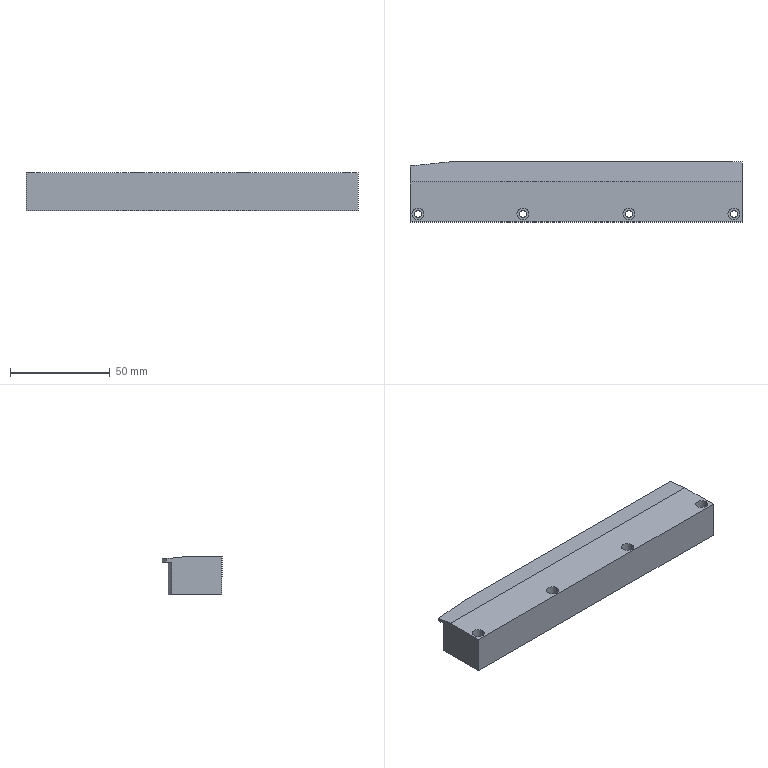Part | SolidWorks | features BaseBody 1 | 1 solid | 31 faces | box 166 x 30 x 19 mm | volume 83734 mm3 | cylinder 16 | plane 15 | commonest cylinder face diameters 3.5 x8 6 x8
STEP:
#1=CARTESIAN_POINT('',(112.721,-3.095,0.));
#2=VERTEX_POINT('',#1);
#3=CARTESIAN_POINT('',(109.221,-3.095,0.));
#4=VERTEX_POINT('',#3);
#5=CARTESIAN_POINT('',(110.971,-3.095,0.));
#6=DIRECTION('',(0.,0.,-1.));
#7=DIRECTION('',(1.,0.,0.));
#8=AXIS2_PLACEMENT_3D('',#5,#6,#7);
#9=CIRCLE('',#8,1.75);
#10=EDGE_CURVE('',#2,#4,#9,.T.);
#11=ORIENTED_EDGE('',*,*,#10,.T.);
#12=CARTESIAN_POINT('',(109.221,-3.095,9.));
#13=VERTEX_POINT('',#12);
#14=CARTESIAN_POINT('',(109.221,-3.095,-150.756));
#15=DIRECTION('',(0.,0.,1.));
#16=VECTOR('',#15,1000.);
#17=LINE('',#14,#16);
#18=EDGE_CURVE('',#4,#13,#17,.T.);
#19=ORIENTED_EDGE('',*,*,#18,.T.);
#20=CARTESIAN_POINT('',(112.721,-3.095,9.));
#21=VERTEX_POINT('',#20);
#22=CARTESIAN_POINT('',(110.971,-3.095,9.));
#23=DIRECTION('',(0.,0.,-1.));
#24=DIRECTION('',(1.,0.,0.));
#25=AXIS2_PLACEMENT_3D('',#22,#23,#24);
#26=CIRCLE('',#25,1.75);
#27=EDGE_CURVE('',#21,#13,#26,.T.);
#28=ORIENTED_EDGE('',*,*,#27,.F.);
#29=CARTESIAN_POINT('',(112.721,-3.095,-150.756));
#30=DIRECTION('',(0.,0.,1.));
#31=VECTOR('',#30,1000.);
#32=LINE('',#29,#31);
#33=EDGE_CURVE('',#2,#21,#32,.T.);
#34=ORIENTED_EDGE('',*,*,#33,.F.);
#35=EDGE_LOOP('',(#11,#19,#28,#34));
#36=FACE_OUTER_BOUND('',#35,.T.);
#37=CARTESIAN_POINT('',(110.971,-3.095,-150.756));
#38=DIRECTION('',(0.,0.,1.));
#39=DIRECTION('',(1.,0.,0.));
#40=AXIS2_PLACEMENT_3D('',#37,#38,#39);
#41=CYLINDRICAL_SURFACE('',#40,1.75);
#42=ADVANCED_FACE('',(#36),#41,.F.);
#43=CARTESIAN_POINT('',(60.221,-3.095,0.));
#44=VERTEX_POINT('',#43);
#45=CARTESIAN_POINT('',(56.721,-3.095,0.));
#46=VERTEX_POINT('',#45);
#47=CARTESIAN_POINT('',(58.471,-3.095,0.));
#48=DIRECTION('',(0.,0.,-1.));
#49=DIRECTION('',(1.,0.,0.));
#50=AXIS2_PLACEMENT_3D('',#47,#48,#49);
#51=CIRCLE('',#50,1.75);
#52=EDGE_CURVE('',#44,#46,#51,.T.);
#53=ORIENTED_EDGE('',*,*,#52,.T.);
#54=CARTESIAN_POINT('',(56.721,-3.095,9.));
#55=VERTEX_POINT('',#54);
#56=CARTESIAN_POINT('',(56.721,-3.095,-150.756));
#57=DIRECTION('',(0.,0.,1.));
#58=VECTOR('',#57,1000.);
#59=LINE('',#56,#58);
#60=EDGE_CURVE('',#46,#55,#59,.T.);
#61=ORIENTED_EDGE('',*,*,#60,.T.);
#62=CARTESIAN_POINT('',(60.221,-3.095,9.));
#63=VERTEX_POINT('',#62);
#64=CARTESIAN_POINT('',(58.471,-3.095,9.));
#65=DIRECTION('',(0.,0.,-1.));
#66=DIRECTION('',(1.,0.,0.));
#67=AXIS2_PLACEMENT_3D('',#64,#65,#66);
#68=CIRCLE('',#67,1.75);
#69=EDGE_CURVE('',#63,#55,#68,.T.);
#70=ORIENTED_EDGE('',*,*,#69,.F.);
#71=CARTESIAN_POINT('',(60.221,-3.095,-150.756));
#72=DIRECTION('',(0.,0.,1.));
#73=VECTOR('',#72,1000.);
#74=LINE('',#71,#73);
#75=EDGE_CURVE('',#44,#63,#74,.T.);
#76=ORIENTED_EDGE('',*,*,#75,.F.);
#77=EDGE_LOOP('',(#53,#61,#70,#76));
#78=FACE_OUTER_BOUND('',#77,.T.);
#79=CARTESIAN_POINT('',(58.471,-3.095,-150.756));
#80=DIRECTION('',(0.,0.,1.));
#81=DIRECTION('',(1.,0.,0.));
#82=AXIS2_PLACEMENT_3D('',#79,#80,#81);
#83=CYLINDRICAL_SURFACE('',#82,1.75);
#84=ADVANCED_FACE('',(#78),#83,.F.);
#85=CARTESIAN_POINT('',(7.221,-3.095,0.));
#86=VERTEX_POINT('',#85);
#87=CARTESIAN_POINT('',(3.721,-3.095,0.));
#88=VERTEX_POINT('',#87);
#89=CARTESIAN_POINT('',(5.471,-3.095,0.));
#90=DIRECTION('',(0.,0.,-1.));
#91=DIRECTION('',(1.,0.,0.));
#92=AXIS2_PLACEMENT_3D('',#89,#90,#91);
#93=CIRCLE('',#92,1.75);
#94=EDGE_CURVE('',#86,#88,#93,.T.);
#95=ORIENTED_EDGE('',*,*,#94,.T.);
#96=CARTESIAN_POINT('',(3.721,-3.095,9.));
#97=VERTEX_POINT('',#96);
#98=CARTESIAN_POINT('',(3.721,-3.095,-150.756));
#99=DIRECTION('',(0.,0.,1.));
#100=VECTOR('',#99,1000.);
#101=LINE('',#98,#100);
#102=EDGE_CURVE('',#88,#97,#101,.T.);
#103=ORIENTED_EDGE('',*,*,#102,.T.);
#104=CARTESIAN_POINT('',(7.221,-3.095,9.));
#105=VERTEX_POINT('',#104);
#106=CARTESIAN_POINT('',(5.471,-3.095,9.));
#107=DIRECTION('',(0.,0.,-1.));
#108=DIRECTION('',(1.,0.,0.));
#109=AXIS2_PLACEMENT_3D('',#106,#107,#108);
#110=CIRCLE('',#109,1.75);
#111=EDGE_CURVE('',#105,#97,#110,.T.);
#112=ORIENTED_EDGE('',*,*,#111,.F.);
#113=CARTESIAN_POINT('',(7.221,-3.095,-150.756));
#114=DIRECTION('',(0.,0.,1.));
#115=VECTOR('',#114,1000.);
#116=LINE('',#113,#115);
#117=EDGE_CURVE('',#86,#105,#116,.T.);
#118=ORIENTED_EDGE('',*,*,#117,.F.);
#119=EDGE_LOOP('',(#95,#103,#112,#118));
#120=FACE_OUTER_BOUND('',#119,.T.);
#121=CARTESIAN_POINT('',(5.471,-3.095,-150.756));
#122=DIRECTION('',(0.,0.,1.));
#123=DIRECTION('',(1.,0.,0.));
#124=AXIS2_PLACEMENT_3D('',#121,#122,#123);
#125=CYLINDRICAL_SURFACE('',#124,1.75);
#126=ADVANCED_FACE('',(#120),#125,.F.);
#127=CARTESIAN_POINT('',(-45.279,-3.095,0.));
#128=VERTEX_POINT('',#127);
#129=CARTESIAN_POINT('',(-48.779,-3.095,0.));
#130=VERTEX_POINT('',#129);
#131=CARTESIAN_POINT('',(-47.029,-3.095,0.));
#132=DIRECTION('',(0.,0.,-1.));
#133=DIRECTION('',(1.,0.,0.));
#134=AXIS2_PLACEMENT_3D('',#131,#132,#133);
#135=CIRCLE('',#134,1.75);
#136=EDGE_CURVE('',#128,#130,#135,.T.);
#137=ORIENTED_EDGE('',*,*,#136,.T.);
#138=CARTESIAN_POINT('',(-48.779,-3.095,9.));
#139=VERTEX_POINT('',#138);
#140=CARTESIAN_POINT('',(-48.779,-3.095,-150.756));
#141=DIRECTION('',(0.,0.,1.));
#142=VECTOR('',#141,1000.);
#143=LINE('',#140,#142);
#144=EDGE_CURVE('',#130,#139,#143,.T.);
#145=ORIENTED_EDGE('',*,*,#144,.T.);
#146=CARTESIAN_POINT('',(-45.279,-3.095,9.));
#147=VERTEX_POINT('',#146);
#148=CARTESIAN_POINT('',(-47.029,-3.095,9.));
#149=DIRECTION('',(0.,0.,-1.));
#150=DIRECTION('',(1.,0.,0.));
#151=AXIS2_PLACEMENT_3D('',#148,#149,#150);
#152=CIRCLE('',#151,1.75);
#153=EDGE_CURVE('',#147,#139,#152,.T.);
#154=ORIENTED_EDGE('',*,*,#153,.F.);
#155=CARTESIAN_POINT('',(-45.279,-3.095,-150.756));
#156=DIRECTION('',(0.,0.,1.));
#157=VECTOR('',#156,1000.);
#158=LINE('',#155,#157);
#159=EDGE_CURVE('',#128,#147,#158,.T.);
#160=ORIENTED_EDGE('',*,*,#159,.F.);
#161=EDGE_LOOP('',(#137,#145,#154,#160));
#162=FACE_OUTER_BOUND('',#161,.T.);
#163=CARTESIAN_POINT('',(-47.029,-3.095,-150.756));
#164=DIRECTION('',(0.,0.,1.));
#165=DIRECTION('',(1.,0.,0.));
#166=AXIS2_PLACEMENT_3D('',#163,#164,#165);
#167=CYLINDRICAL_SURFACE('',#166,1.75);
#168=ADVANCED_FACE('',(#162),#167,.F.);
#169=CARTESIAN_POINT('',(107.971,-3.095,9.));
#170=VERTEX_POINT('',#169);
#171=CARTESIAN_POINT('',(113.971,-3.095,9.));
#172=VERTEX_POINT('',#171);
#173=CARTESIAN_POINT('',(110.971,-3.095,9.));
#174=DIRECTION('',(0.,0.,1.));
#175=DIRECTION('',(1.,0.,0.));
#176=AXIS2_PLACEMENT_3D('',#173,#174,#175);
#177=CIRCLE('',#176,3.);
#178=EDGE_CURVE('',#170,#172,#177,.T.);
#179=ORIENTED_EDGE('',*,*,#178,.F.);
#180=CARTESIAN_POINT('',(107.971,-3.095,19.));
#181=VERTEX_POINT('',#180);
#182=CARTESIAN_POINT('',(107.971,-3.095,14.));
#183=DIRECTION('',(0.,0.,1.));
#184=VECTOR('',#183,1000.);
#185=LINE('',#182,#184);
#186=EDGE_CURVE('',#170,#181,#185,.T.);
#187=ORIENTED_EDGE('',*,*,#186,.T.);
#188=CARTESIAN_POINT('',(113.971,-3.095,19.));
#189=VERTEX_POINT('',#188);
#190=CARTESIAN_POINT('',(110.971,-3.095,19.));
#191=DIRECTION('',(0.,0.,-1.));
#192=DIRECTION('',(1.,0.,0.));
#193=AXIS2_PLACEMENT_3D('',#190,#191,#192);
#194=CIRCLE('',#193,3.);
#195=EDGE_CURVE('',#189,#181,#194,.T.);
#196=ORIENTED_EDGE('',*,*,#195,.F.);
#197=CARTESIAN_POINT('',(113.971,-3.095,14.));
#198=DIRECTION('',(0.,0.,1.));
#199=VECTOR('',#198,1000.);
#200=LINE('',#197,#199);
#201=EDGE_CURVE('',#172,#189,#200,.T.);
#202=ORIENTED_EDGE('',*,*,#201,.F.);
#203=EDGE_LOOP('',(#179,#187,#196,#202));
#204=FACE_OUTER_BOUND('',#203,.T.);
#205=CARTESIAN_POINT('',(110.971,-3.095,14.));
#206=DIRECTION('',(0.,0.,1.));
#207=DIRECTION('',(1.,0.,0.));
#208=AXIS2_PLACEMENT_3D('',#205,#206,#207);
#209=CYLINDRICAL_SURFACE('',#208,3.);
#210=ADVANCED_FACE('',(#204),#209,.F.);
#211=CARTESIAN_POINT('',(55.471,-3.095,9.));
#212=VERTEX_POINT('',#211);
#213=CARTESIAN_POINT('',(61.471,-3.095,9.));
#214=VERTEX_POINT('',#213);
#215=CARTESIAN_POINT('',(58.471,-3.095,9.));
#216=DIRECTION('',(0.,0.,1.));
#217=DIRECTION('',(1.,0.,0.));
#218=AXIS2_PLACEMENT_3D('',#215,#216,#217);
#219=CIRCLE('',#218,3.);
#220=EDGE_CURVE('',#212,#214,#219,.T.);
#221=ORIENTED_EDGE('',*,*,#220,.F.);
#222=CARTESIAN_POINT('',(55.471,-3.095,19.));
#223=VERTEX_POINT('',#222);
#224=CARTESIAN_POINT('',(55.471,-3.095,14.));
#225=DIRECTION('',(0.,0.,1.));
#226=VECTOR('',#225,1000.);
#227=LINE('',#224,#226);
#228=EDGE_CURVE('',#212,#223,#227,.T.);
#229=ORIENTED_EDGE('',*,*,#228,.T.);
#230=CARTESIAN_POINT('',(61.471,-3.095,19.));
#231=VERTEX_POINT('',#230);
#232=CARTESIAN_POINT('',(58.471,-3.095,19.));
#233=DIRECTION('',(0.,0.,-1.));
#234=DIRECTION('',(1.,0.,0.));
#235=AXIS2_PLACEMENT_3D('',#232,#233,#234);
#236=CIRCLE('',#235,3.);
#237=EDGE_CURVE('',#231,#223,#236,.T.);
#238=ORIENTED_EDGE('',*,*,#237,.F.);
#239=CARTESIAN_POINT('',(61.471,-3.095,14.));
#240=DIRECTION('',(0.,0.,1.));
#241=VECTOR('',#240,1000.);
#242=LINE('',#239,#241);
#243=EDGE_CURVE('',#214,#231,#242,.T.);
#244=ORIENTED_EDGE('',*,*,#243,.F.);
#245=EDGE_LOOP('',(#221,#229,#238,#244));
#246=FACE_OUTER_BOUND('',#245,.T.);
#247=CARTESIAN_POINT('',(58.471,-3.095,14.));
#248=DIRECTION('',(0.,0.,1.));
#249=DIRECTION('',(1.,0.,0.));
#250=AXIS2_PLACEMENT_3D('',#247,#248,#249);
#251=CYLINDRICAL_SURFACE('',#250,3.);
#252=ADVANCED_FACE('',(#246),#251,.F.);
#253=CARTESIAN_POINT('',(2.471,-3.095,9.));
#254=VERTEX_POINT('',#253);
#255=CARTESIAN_POINT('',(8.471,-3.095,9.));
#256=VERTEX_POINT('',#255);
#257=CARTESIAN_POINT('',(5.471,-3.095,9.));
#258=DIRECTION('',(0.,0.,1.));
#259=DIRECTION('',(1.,0.,0.));
#260=AXIS2_PLACEMENT_3D('',#257,#258,#259);
#261=CIRCLE('',#260,3.);
#262=EDGE_CURVE('',#254,#256,#261,.T.);
#263=ORIENTED_EDGE('',*,*,#262,.F.);
#264=CARTESIAN_POINT('',(2.471,-3.095,19.));
#265=VERTEX_POINT('',#264);
#266=CARTESIAN_POINT('',(2.471,-3.095,14.));
#267=DIRECTION('',(0.,0.,1.));
#268=VECTOR('',#267,1000.);
#269=LINE('',#266,#268);
#270=EDGE_CURVE('',#254,#265,#269,.T.);
#271=ORIENTED_EDGE('',*,*,#270,.T.);
#272=CARTESIAN_POINT('',(8.471,-3.095,19.));
#273=VERTEX_POINT('',#272);
#274=CARTESIAN_POINT('',(5.471,-3.095,19.));
#275=DIRECTION('',(0.,0.,-1.));
#276=DIRECTION('',(1.,0.,0.));
#277=AXIS2_PLACEMENT_3D('',#274,#275,#276);
#278=CIRCLE('',#277,3.);
#279=EDGE_CURVE('',#273,#265,#278,.T.);
#280=ORIENTED_EDGE('',*,*,#279,.F.);
#281=CARTESIAN_POINT('',(8.471,-3.095,14.));
#282=DIRECTION('',(0.,0.,1.));
#283=VECTOR('',#282,1000.);
#284=LINE('',#281,#283);
#285=EDGE_CURVE('',#256,#273,#284,.T.);
#286=ORIENTED_EDGE('',*,*,#285,.F.);
#287=EDGE_LOOP('',(#263,#271,#280,#286));
#288=FACE_OUTER_BOUND('',#287,.T.);
#289=CARTESIAN_POINT('',(5.471,-3.095,14.));
#290=DIRECTION('',(0.,0.,1.));
#291=DIRECTION('',(1.,0.,0.));
#292=AXIS2_PLACEMENT_3D('',#289,#290,#291);
#293=CYLINDRICAL_SURFACE('',#292,3.);
#294=ADVANCED_FACE('',(#288),#293,.F.);
#295=CARTESIAN_POINT('',(-50.029,-3.095,9.));
#296=VERTEX_POINT('',#295);
#297=CARTESIAN_POINT('',(-44.029,-3.095,9.));
#298=VERTEX_POINT('',#297);
#299=CARTESIAN_POINT('',(-47.029,-3.095,9.));
#300=DIRECTION('',(0.,0.,1.));
#301=DIRECTION('',(1.,0.,0.));
#302=AXIS2_PLACEMENT_3D('',#299,#300,#301);
#303=CIRCLE('',#302,3.);
#304=EDGE_CURVE('',#296,#298,#303,.T.);
#305=ORIENTED_EDGE('',*,*,#304,.F.);
#306=CARTESIAN_POINT('',(-50.029,-3.095,19.));
#307=VERTEX_POINT('',#306);
#308=CARTESIAN_POINT('',(-50.029,-3.095,14.));
#309=DIRECTION('',(0.,0.,1.));
#310=VECTOR('',#309,1000.);
#311=LINE('',#308,#310);
#312=EDGE_CURVE('',#296,#307,#311,.T.);
#313=ORIENTED_EDGE('',*,*,#312,.T.);
#314=CARTESIAN_POINT('',(-44.029,-3.095,19.));
#315=VERTEX_POINT('',#314);
#316=CARTESIAN_POINT('',(-47.029,-3.095,19.));
#317=DIRECTION('',(0.,0.,-1.));
#318=DIRECTION('',(1.,0.,0.));
#319=AXIS2_PLACEMENT_3D('',#316,#317,#318);
#320=CIRCLE('',#319,3.);
#321=EDGE_CURVE('',#315,#307,#320,.T.);
#322=ORIENTED_EDGE('',*,*,#321,.F.);
#323=CARTESIAN_POINT('',(-44.029,-3.095,14.));
#324=DIRECTION('',(0.,0.,1.));
#325=VECTOR('',#324,1000.);
#326=LINE('',#323,#325);
#327=EDGE_CURVE('',#298,#315,#326,.T.);
#328=ORIENTED_EDGE('',*,*,#327,.F.);
#329=EDGE_LOOP('',(#305,#313,#322,#328));
#330=FACE_OUTER_BOUND('',#329,.T.);
#331=CARTESIAN_POINT('',(-47.029,-3.095,14.));
#332=DIRECTION('',(0.,0.,1.));
#333=DIRECTION('',(1.,0.,0.));
#334=AXIS2_PLACEMENT_3D('',#331,#332,#333);
#335=CYLINDRICAL_SURFACE('',#334,3.);
#336=ADVANCED_FACE('',(#330),#335,.F.);
#337=ORIENTED_EDGE('',*,*,#10,.F.);
#338=CARTESIAN_POINT('',(110.971,-3.095,0.));
#339=DIRECTION('',(0.,0.,-1.));
#340=DIRECTION('',(1.,0.,0.));
#341=AXIS2_PLACEMENT_3D('',#338,#339,#340);
#342=CIRCLE('',#341,1.75);
#343=EDGE_CURVE('',#4,#2,#342,.T.);
#344=ORIENTED_EDGE('',*,*,#343,.F.);
#345=EDGE_LOOP('',(#337,#344));
#346=FACE_BOUND('',#345,.T.);
#347=ORIENTED_EDGE('',*,*,#52,.F.);
#348=CARTESIAN_POINT('',(58.471,-3.095,0.));
#349=DIRECTION('',(0.,0.,-1.));
#350=DIRECTION('',(1.,0.,0.));
#351=AXIS2_PLACEMENT_3D('',#348,#349,#350);
#352=CIRCLE('',#351,1.75);
#353=EDGE_CURVE('',#46,#44,#352,.T.);
#354=ORIENTED_EDGE('',*,*,#353,.F.);
#355=EDGE_LOOP('',(#347,#354));
#356=FACE_BOUND('',#355,.T.);
#357=ORIENTED_EDGE('',*,*,#94,.F.);
#358=CARTESIAN_POINT('',(5.471,-3.095,0.));
#359=DIRECTION('',(0.,0.,-1.));
#360=DIRECTION('',(1.,0.,0.));
#361=AXIS2_PLACEMENT_3D('',#358,#359,#360);
#362=CIRCLE('',#361,1.75);
#363=EDGE_CURVE('',#88,#86,#362,.T.);
#364=ORIENTED_EDGE('',*,*,#363,.F.);
#365=EDGE_LOOP('',(#357,#364));
#366=FACE_BOUND('',#365,.T.);
#367=ORIENTED_EDGE('',*,*,#136,.F.);
#368=CARTESIAN_POINT('',(-47.029,-3.095,0.));
#369=DIRECTION('',(0.,0.,-1.));
#370=DIRECTION('',(1.,0.,0.));
#371=AXIS2_PLACEMENT_3D('',#368,#369,#370);
#372=CIRCLE('',#371,1.75);
#373=EDGE_CURVE('',#130,#128,#372,.T.);
#374=ORIENTED_EDGE('',*,*,#373,.F.);
#375=EDGE_LOOP('',(#367,#374));
#376=FACE_BOUND('',#375,.T.);
#377=CARTESIAN_POINT('',(114.971,19.905,0.));
#378=VERTEX_POINT('',#377);
#379=CARTESIAN_POINT('',(-31.029,19.905,0.));
#380=VERTEX_POINT('',#379);
#381=CARTESIAN_POINT('',(31.971,19.905,0.));
#382=DIRECTION('',(-1.,0.,0.));
#383=VECTOR('',#382,1000.);
#384=LINE('',#381,#383);
#385=EDGE_CURVE('',#378,#380,#384,.T.);
#386=ORIENTED_EDGE('',*,*,#385,.F.);
#387=CARTESIAN_POINT('',(114.971,-7.095,0.));
#388=VERTEX_POINT('',#387);
#389=CARTESIAN_POINT('',(114.971,7.905,0.));
#390=DIRECTION('',(0.,1.,0.));
#391=VECTOR('',#390,1000.);
#392=LINE('',#389,#391);
#393=EDGE_CURVE('',#388,#378,#392,.T.);
#394=ORIENTED_EDGE('',*,*,#393,.F.);
#395=CARTESIAN_POINT('',(-51.029,-7.095,0.));
#396=VERTEX_POINT('',#395);
#397=CARTESIAN_POINT('',(31.971,-7.095,0.));
#398=DIRECTION('',(1.,0.,0.));
#399=VECTOR('',#398,1000.);
#400=LINE('',#397,#399);
#401=EDGE_CURVE('',#396,#388,#400,.T.);
#402=ORIENTED_EDGE('',*,*,#401,.F.);
#403=CARTESIAN_POINT('',(-51.029,17.905,0.));
#404=VERTEX_POINT('',#403);
#405=CARTESIAN_POINT('',(-51.029,7.905,0.));
#406=DIRECTION('',(0.,-1.,0.));
#407=VECTOR('',#406,1000.);
#408=LINE('',#405,#407);
#409=EDGE_CURVE('',#404,#396,#408,.T.);
#410=ORIENTED_EDGE('',*,*,#409,.F.);
#411=CARTESIAN_POINT('',(-31.029,19.905,0.));
#412=DIRECTION('',(-0.995,-0.0995,0.));
#413=VECTOR('',#412,1000.);
#414=LINE('',#411,#413);
#415=EDGE_CURVE('',#380,#404,#414,.T.);
#416=ORIENTED_EDGE('',*,*,#415,.F.);
#417=EDGE_LOOP('',(#386,#394,#402,#410,#416));
#418=FACE_OUTER_BOUND('',#417,.T.);
#419=CARTESIAN_POINT('',(31.971,7.905,0.));
#420=DIRECTION('',(0.,0.,1.));
#421=DIRECTION('',(1.,0.,0.));
#422=AXIS2_PLACEMENT_3D('',#419,#420,#421);
#423=PLANE('',#422);
#424=ADVANCED_FACE('',(#346,#356,#366,#376,#418),#423,.F.);
#425=ORIENTED_EDGE('',*,*,#18,.F.);
#426=ORIENTED_EDGE('',*,*,#343,.T.);
#427=ORIENTED_EDGE('',*,*,#33,.T.);
#428=CARTESIAN_POINT('',(110.971,-3.095,9.));
#429=DIRECTION('',(0.,0.,-1.));
#430=DIRECTION('',(1.,0.,0.));
#431=AXIS2_PLACEMENT_3D('',#428,#429,#430);
#432=CIRCLE('',#431,1.75);
#433=EDGE_CURVE('',#13,#21,#432,.T.);
#434=ORIENTED_EDGE('',*,*,#433,.F.);
#435=EDGE_LOOP('',(#425,#426,#427,#434));
#436=FACE_OUTER_BOUND('',#435,.T.);
#437=CARTESIAN_POINT('',(110.971,-3.095,-150.756));
#438=DIRECTION('',(0.,0.,1.));
#439=DIRECTION('',(1.,0.,0.));
#440=AXIS2_PLACEMENT_3D('',#437,#438,#439);
#441=CYLINDRICAL_SURFACE('',#440,1.75);
#442=ADVANCED_FACE('',(#436),#441,.F.);
#443=ORIENTED_EDGE('',*,*,#60,.F.);
#444=ORIENTED_EDGE('',*,*,#353,.T.);
#445=ORIENTED_EDGE('',*,*,#75,.T.);
#446=CARTESIAN_POINT('',(58.471,-3.095,9.));
#447=DIRECTION('',(0.,0.,-1.));
#448=DIRECTION('',(1.,0.,0.));
#449=AXIS2_PLACEMENT_3D('',#446,#447,#448);
#450=CIRCLE('',#449,1.75);
#451=EDGE_CURVE('',#55,#63,#450,.T.);
#452=ORIENTED_EDGE('',*,*,#451,.F.);
#453=EDGE_LOOP('',(#443,#444,#445,#452));
#454=FACE_OUTER_BOUND('',#453,.T.);
#455=CARTESIAN_POINT('',(58.471,-3.095,-150.756));
#456=DIRECTION('',(0.,0.,1.));
#457=DIRECTION('',(1.,0.,0.));
#458=AXIS2_PLACEMENT_3D('',#455,#456,#457);
#459=CYLINDRICAL_SURFACE('',#458,1.75);
#460=ADVANCED_FACE('',(#454),#459,.F.);
#461=ORIENTED_EDGE('',*,*,#102,.F.);
#462=ORIENTED_EDGE('',*,*,#363,.T.);
#463=ORIENTED_EDGE('',*,*,#117,.T.);
#464=CARTESIAN_POINT('',(5.471,-3.095,9.));
#465=DIRECTION('',(0.,0.,-1.));
#466=DIRECTION('',(1.,0.,0.));
#467=AXIS2_PLACEMENT_3D('',#464,#465,#466);
#468=CIRCLE('',#467,1.75);
#469=EDGE_CURVE('',#97,#105,#468,.T.);
#470=ORIENTED_EDGE('',*,*,#469,.F.);
#471=EDGE_LOOP('',(#461,#462,#463,#470));
#472=FACE_OUTER_BOUND('',#471,.T.);
#473=CARTESIAN_POINT('',(5.471,-3.095,-150.756));
#474=DIRECTION('',(0.,0.,1.));
#475=DIRECTION('',(1.,0.,0.));
#476=AXIS2_PLACEMENT_3D('',#473,#474,#475);
#477=CYLINDRICAL_SURFACE('',#476,1.75);
#478=ADVANCED_FACE('',(#472),#477,.F.);
#479=ORIENTED_EDGE('',*,*,#144,.F.);
#480=ORIENTED_EDGE('',*,*,#373,.T.);
#481=ORIENTED_EDGE('',*,*,#159,.T.);
#482=CARTESIAN_POINT('',(-47.029,-3.095,9.));
#483=DIRECTION('',(0.,0.,-1.));
#484=DIRECTION('',(1.,0.,0.));
#485=AXIS2_PLACEMENT_3D('',#482,#483,#484);
#486=CIRCLE('',#485,1.75);
#487=EDGE_CURVE('',#139,#147,#486,.T.);
#488=ORIENTED_EDGE('',*,*,#487,.F.);
#489=EDGE_LOOP('',(#479,#480,#481,#488));
#490=FACE_OUTER_BOUND('',#489,.T.);
#491=CARTESIAN_POINT('',(-47.029,-3.095,-150.756));
#492=DIRECTION('',(0.,0.,1.));
#493=DIRECTION('',(1.,0.,0.));
#494=AXIS2_PLACEMENT_3D('',#491,#492,#493);
#495=CYLINDRICAL_SURFACE('',#494,1.75);
#496=ADVANCED_FACE('',(#490),#495,.F.);
#497=CARTESIAN_POINT('',(-51.029,17.905,16.5));
#498=VERTEX_POINT('',#497);
#499=CARTESIAN_POINT('',(-31.029,19.905,16.5));
#500=VERTEX_POINT('',#499);
#501=CARTESIAN_POINT('',(-41.029,18.905,16.5));
#502=DIRECTION('',(0.995,0.0995,0.));
#503=VECTOR('',#502,1000.);
#504=LINE('',#501,#503);
#505=EDGE_CURVE('',#498,#500,#504,.T.);
#506=ORIENTED_EDGE('',*,*,#505,.T.);
#507=CARTESIAN_POINT('',(-31.029,19.905,0.));
#508=DIRECTION('',(0.,0.,-1.));
#509=VECTOR('',#508,1000.);
#510=LINE('',#507,#509);
#511=EDGE_CURVE('',#500,#380,#510,.T.);
#512=ORIENTED_EDGE('',*,*,#511,.T.);
#513=ORIENTED_EDGE('',*,*,#415,.T.);
#514=CARTESIAN_POINT('',(-51.029,17.905,0.));
#515=DIRECTION('',(0.,0.,1.));
#516=VECTOR('',#515,1000.);
#517=LINE('',#514,#516);
#518=EDGE_CURVE('',#404,#498,#517,.T.);
#519=ORIENTED_EDGE('',*,*,#518,.T.);
#520=EDGE_LOOP('',(#506,#512,#513,#519));
#521=FACE_OUTER_BOUND('',#520,.T.);
#522=CARTESIAN_POINT('',(-41.029,18.905,0.));
#523=DIRECTION('',(-0.0995,0.995,0.));
#524=DIRECTION('',(-0.995,-0.0995,0.));
#525=AXIS2_PLACEMENT_3D('',#522,#523,#524);
#526=PLANE('',#525);
#527=ADVANCED_FACE('',(#521),#526,.T.);
#528=CARTESIAN_POINT('',(114.971,19.905,16.5));
#529=VERTEX_POINT('',#528);
#530=CARTESIAN_POINT('',(114.971,19.905,16.5));
#531=DIRECTION('',(-1.,0.,0.));
#532=VECTOR('',#531,1000.);
#533=LINE('',#530,#532);
#534=EDGE_CURVE('',#529,#500,#533,.T.);
#535=ORIENTED_EDGE('',*,*,#534,.F.);
#536=CARTESIAN_POINT('',(114.971,19.905,0.));
#537=DIRECTION('',(0.,0.,1.));
#538=VECTOR('',#537,1000.);
#539=LINE('',#536,#538);
#540=EDGE_CURVE('',#378,#529,#539,.T.);
#541=ORIENTED_EDGE('',*,*,#540,.F.);
#542=ORIENTED_EDGE('',*,*,#385,.T.);
#543=ORIENTED_EDGE('',*,*,#511,.F.);
#544=EDGE_LOOP('',(#535,#541,#542,#543));
#545=FACE_OUTER_BOUND('',#544,.T.);
#546=CARTESIAN_POINT('',(114.971,19.905,0.));
#547=DIRECTION('',(0.,-1.,0.));
#548=DIRECTION('',(0.,0.,-1.));
#549=AXIS2_PLACEMENT_3D('',#546,#547,#548);
#550=PLANE('',#549);
#551=ADVANCED_FACE('',(#545),#550,.F.);
#552=CARTESIAN_POINT('',(114.971,22.905,16.5));
#553=VERTEX_POINT('',#552);
#554=CARTESIAN_POINT('',(114.971,22.905,16.5));
#555=DIRECTION('',(0.,1.,0.));
#556=VECTOR('',#555,1000.);
#557=LINE('',#554,#556);
#558=EDGE_CURVE('',#529,#553,#557,.T.);
#559=ORIENTED_EDGE('',*,*,#558,.T.);
#560=CARTESIAN_POINT('',(114.971,22.905,18.));
#561=VERTEX_POINT('',#560);
#562=CARTESIAN_POINT('',(114.971,22.905,0.));
#563=DIRECTION('',(0.,0.,-1.));
#564=VECTOR('',#563,1000.);
#565=LINE('',#562,#564);
#566=EDGE_CURVE('',#561,#553,#565,.T.);
#567=ORIENTED_EDGE('',*,*,#566,.F.);
#568=CARTESIAN_POINT('',(114.971,12.905,19.));
#569=VERTEX_POINT('',#568);
#570=CARTESIAN_POINT('',(114.971,22.905,18.));
#571=DIRECTION('',(0.,-0.995,0.0995));
#572=VECTOR('',#571,1000.);
#573=LINE('',#570,#572);
#574=EDGE_CURVE('',#561,#569,#573,.T.);
#575=ORIENTED_EDGE('',*,*,#574,.T.);
#576=CARTESIAN_POINT('',(114.971,-7.095,19.));
#577=VERTEX_POINT('',#576);
#578=CARTESIAN_POINT('',(114.971,22.905,19.));
#579=DIRECTION('',(0.,-1.,0.));
#580=VECTOR('',#579,1000.);
#581=LINE('',#578,#580);
#582=EDGE_CURVE('',#569,#577,#581,.T.);
#583=ORIENTED_EDGE('',*,*,#582,.T.);
#584=CARTESIAN_POINT('',(114.971,-7.095,0.));
#585=DIRECTION('',(0.,0.,-1.));
#586=VECTOR('',#585,1000.);
#587=LINE('',#584,#586);
#588=EDGE_CURVE('',#577,#388,#587,.T.);
#589=ORIENTED_EDGE('',*,*,#588,.T.);
#590=ORIENTED_EDGE('',*,*,#393,.T.);
#591=ORIENTED_EDGE('',*,*,#540,.T.);
#592=EDGE_LOOP('',(#559,#567,#575,#583,#589,#590,#591));
#593=FACE_OUTER_BOUND('',#592,.T.);
#594=CARTESIAN_POINT('',(114.971,22.905,0.));
#595=DIRECTION('',(1.,0.,0.));
#596=DIRECTION('',(0.,0.,-1.));
#597=AXIS2_PLACEMENT_3D('',#594,#595,#596);
#598=PLANE('',#597);
#599=ADVANCED_FACE('',(#593),#598,.T.);
#600=ORIENTED_EDGE('',*,*,#401,.T.);
#601=ORIENTED_EDGE('',*,*,#588,.F.);
#602=CARTESIAN_POINT('',(-51.029,-7.095,19.));
#603=VERTEX_POINT('',#602);
#604=CARTESIAN_POINT('',(114.971,-7.095,19.));
#605=DIRECTION('',(-1.,0.,0.));
#606=VECTOR('',#605,1000.);
#607=LINE('',#604,#606);
#608=EDGE_CURVE('',#577,#603,#607,.T.);
#609=ORIENTED_EDGE('',*,*,#608,.T.);
#610=CARTESIAN_POINT('',(-51.029,-7.095,0.));
#611=DIRECTION('',(0.,0.,-1.));
#612=VECTOR('',#611,1000.);
#613=LINE('',#610,#612);
#614=EDGE_CURVE('',#603,#396,#613,.T.);
#615=ORIENTED_EDGE('',*,*,#614,.T.);
#616=EDGE_LOOP('',(#600,#601,#609,#615));
#617=FACE_OUTER_BOUND('',#616,.T.);
#618=CARTESIAN_POINT('',(114.971,-7.095,0.));
#619=DIRECTION('',(0.,-1.,0.));
#620=DIRECTION('',(0.,0.,-1.));
#621=AXIS2_PLACEMENT_3D('',#618,#619,#620);
#622=PLANE('',#621);
#623=ADVANCED_FACE('',(#617),#622,.T.);
#624=CARTESIAN_POINT('',(-51.029,12.905,19.));
#625=VERTEX_POINT('',#624);
#626=CARTESIAN_POINT('',(-51.029,-7.095,19.));
#627=DIRECTION('',(0.,1.,0.));
#628=VECTOR('',#627,1000.);
#629=LINE('',#626,#628);
#630=EDGE_CURVE('',#603,#625,#629,.T.);
#631=ORIENTED_EDGE('',*,*,#630,.T.);
#632=CARTESIAN_POINT('',(-51.029,20.905,18.2));
#633=VERTEX_POINT('',#632);
#634=CARTESIAN_POINT('',(-51.029,12.905,19.));
#635=DIRECTION('',(0.,0.995,-0.0995));
#636=VECTOR('',#635,1000.);
#637=LINE('',#634,#636);
#638=EDGE_CURVE('',#625,#633,#637,.T.);
#639=ORIENTED_EDGE('',*,*,#638,.T.);
#640=CARTESIAN_POINT('',(-51.029,20.905,16.5));
#641=VERTEX_POINT('',#640);
#642=CARTESIAN_POINT('',(-51.029,20.905,0.));
#643=DIRECTION('',(0.,0.,1.));
#644=VECTOR('',#643,1000.);
#645=LINE('',#642,#644);
#646=EDGE_CURVE('',#641,#633,#645,.T.);
#647=ORIENTED_EDGE('',*,*,#646,.F.);
#648=CARTESIAN_POINT('',(-51.029,-7.095,16.5));
#649=DIRECTION('',(0.,-1.,0.));
#650=VECTOR('',#649,1000.);
#651=LINE('',#648,#650);
#652=EDGE_CURVE('',#641,#498,#651,.T.);
#653=ORIENTED_EDGE('',*,*,#652,.T.);
#654=ORIENTED_EDGE('',*,*,#518,.F.);
#655=ORIENTED_EDGE('',*,*,#409,.T.);
#656=ORIENTED_EDGE('',*,*,#614,.F.);
#657=EDGE_LOOP('',(#631,#639,#647,#653,#654,#655,#656));
#658=FACE_OUTER_BOUND('',#657,.T.);
#659=CARTESIAN_POINT('',(-51.029,-7.095,0.));
#660=DIRECTION('',(-1.,0.,0.));
#661=DIRECTION('',(0.,0.,1.));
#662=AXIS2_PLACEMENT_3D('',#659,#660,#661);
#663=PLANE('',#662);
#664=ADVANCED_FACE('',(#658),#663,.T.);
#665=ORIENTED_EDGE('',*,*,#27,.T.);
#666=ORIENTED_EDGE('',*,*,#433,.T.);
#667=EDGE_LOOP('',(#665,#666));
#668=FACE_BOUND('',#667,.T.);
#669=CARTESIAN_POINT('',(110.971,-3.095,9.));
#670=DIRECTION('',(0.,0.,1.));
#671=DIRECTION('',(1.,0.,0.));
#672=AXIS2_PLACEMENT_3D('',#669,#670,#671);
#673=CIRCLE('',#672,3.);
#674=EDGE_CURVE('',#172,#170,#673,.T.);
#675=ORIENTED_EDGE('',*,*,#674,.T.);
#676=ORIENTED_EDGE('',*,*,#178,.T.);
#677=EDGE_LOOP('',(#675,#676));
#678=FACE_OUTER_BOUND('',#677,.T.);
#679=CARTESIAN_POINT('',(110.971,-3.095,9.));
#680=DIRECTION('',(0.,0.,1.));
#681=DIRECTION('',(1.,0.,0.));
#682=AXIS2_PLACEMENT_3D('',#679,#680,#681);
#683=PLANE('',#682);
#684=ADVANCED_FACE('',(#668,#678),#683,.T.);
#685=ORIENTED_EDGE('',*,*,#69,.T.);
#686=ORIENTED_EDGE('',*,*,#451,.T.);
#687=EDGE_LOOP('',(#685,#686));
#688=FACE_BOUND('',#687,.T.);
#689=CARTESIAN_POINT('',(58.471,-3.095,9.));
#690=DIRECTION('',(0.,0.,1.));
#691=DIRECTION('',(1.,0.,0.));
#692=AXIS2_PLACEMENT_3D('',#689,#690,#691);
#693=CIRCLE('',#692,3.);
#694=EDGE_CURVE('',#214,#212,#693,.T.);
#695=ORIENTED_EDGE('',*,*,#694,.T.);
#696=ORIENTED_EDGE('',*,*,#220,.T.);
#697=EDGE_LOOP('',(#695,#696));
#698=FACE_OUTER_BOUND('',#697,.T.);
#699=CARTESIAN_POINT('',(58.471,-3.095,9.));
#700=DIRECTION('',(0.,0.,1.));
#701=DIRECTION('',(1.,0.,0.));
#702=AXIS2_PLACEMENT_3D('',#699,#700,#701);
#703=PLANE('',#702);
#704=ADVANCED_FACE('',(#688,#698),#703,.T.);
#705=ORIENTED_EDGE('',*,*,#111,.T.);
#706=ORIENTED_EDGE('',*,*,#469,.T.);
#707=EDGE_LOOP('',(#705,#706));
#708=FACE_BOUND('',#707,.T.);
#709=CARTESIAN_POINT('',(5.471,-3.095,9.));
#710=DIRECTION('',(0.,0.,1.));
#711=DIRECTION('',(1.,0.,0.));
#712=AXIS2_PLACEMENT_3D('',#709,#710,#711);
#713=CIRCLE('',#712,3.);
#714=EDGE_CURVE('',#256,#254,#713,.T.);
#715=ORIENTED_EDGE('',*,*,#714,.T.);
#716=ORIENTED_EDGE('',*,*,#262,.T.);
#717=EDGE_LOOP('',(#715,#716));
#718=FACE_OUTER_BOUND('',#717,.T.);
#719=CARTESIAN_POINT('',(5.471,-3.095,9.));
#720=DIRECTION('',(0.,0.,1.));
#721=DIRECTION('',(1.,0.,0.));
#722=AXIS2_PLACEMENT_3D('',#719,#720,#721);
#723=PLANE('',#722);
#724=ADVANCED_FACE('',(#708,#718),#723,.T.);
#725=ORIENTED_EDGE('',*,*,#153,.T.);
#726=ORIENTED_EDGE('',*,*,#487,.T.);
#727=EDGE_LOOP('',(#725,#726));
#728=FACE_BOUND('',#727,.T.);
#729=CARTESIAN_POINT('',(-47.029,-3.095,9.));
#730=DIRECTION('',(0.,0.,1.));
#731=DIRECTION('',(1.,0.,0.));
#732=AXIS2_PLACEMENT_3D('',#729,#730,#731);
#733=CIRCLE('',#732,3.);
#734=EDGE_CURVE('',#298,#296,#733,.T.);
#735=ORIENTED_EDGE('',*,*,#734,.T.);
#736=ORIENTED_EDGE('',*,*,#304,.T.);
#737=EDGE_LOOP('',(#735,#736));
#738=FACE_OUTER_BOUND('',#737,.T.);
#739=CARTESIAN_POINT('',(-47.029,-3.095,9.));
#740=DIRECTION('',(0.,0.,1.));
#741=DIRECTION('',(1.,0.,0.));
#742=AXIS2_PLACEMENT_3D('',#739,#740,#741);
#743=PLANE('',#742);
#744=ADVANCED_FACE('',(#728,#738),#743,.T.);
#745=CARTESIAN_POINT('',(-31.029,22.905,16.5));
#746=VERTEX_POINT('',#745);
#747=CARTESIAN_POINT('',(31.971,22.905,16.5));
#748=DIRECTION('',(-1.,0.,0.));
#749=VECTOR('',#748,1000.);
#750=LINE('',#747,#749);
#751=EDGE_CURVE('',#553,#746,#750,.T.);
#752=ORIENTED_EDGE('',*,*,#751,.F.);
#753=ORIENTED_EDGE('',*,*,#558,.F.);
#754=ORIENTED_EDGE('',*,*,#534,.T.);
#755=ORIENTED_EDGE('',*,*,#505,.F.);
#756=ORIENTED_EDGE('',*,*,#652,.F.);
#757=CARTESIAN_POINT('',(-31.029,22.905,16.5));
#758=DIRECTION('',(-0.995,-0.0995,0.));
#759=VECTOR('',#758,1000.);
#760=LINE('',#757,#759);
#761=EDGE_CURVE('',#746,#641,#760,.T.);
#762=ORIENTED_EDGE('',*,*,#761,.F.);
#763=EDGE_LOOP('',(#752,#753,#754,#755,#756,#762));
#764=FACE_OUTER_BOUND('',#763,.T.);
#765=CARTESIAN_POINT('',(31.971,21.405,16.5));
#766=DIRECTION('',(0.,0.,1.));
#767=DIRECTION('',(1.,0.,0.));
#768=AXIS2_PLACEMENT_3D('',#765,#766,#767);
#769=PLANE('',#768);
#770=ADVANCED_FACE('',(#764),#769,.F.);
#771=ORIENTED_EDGE('',*,*,#195,.T.);
#772=CARTESIAN_POINT('',(110.971,-3.095,19.));
#773=DIRECTION('',(0.,0.,-1.));
#774=DIRECTION('',(1.,0.,0.));
#775=AXIS2_PLACEMENT_3D('',#772,#773,#774);
#776=CIRCLE('',#775,3.);
#777=EDGE_CURVE('',#181,#189,#776,.T.);
#778=ORIENTED_EDGE('',*,*,#777,.T.);
#779=EDGE_LOOP('',(#771,#778));
#780=FACE_BOUND('',#779,.T.);
#781=ORIENTED_EDGE('',*,*,#237,.T.);
#782=CARTESIAN_POINT('',(58.471,-3.095,19.));
#783=DIRECTION('',(0.,0.,-1.));
#784=DIRECTION('',(1.,0.,0.));
#785=AXIS2_PLACEMENT_3D('',#782,#783,#784);
#786=CIRCLE('',#785,3.);
#787=EDGE_CURVE('',#223,#231,#786,.T.);
#788=ORIENTED_EDGE('',*,*,#787,.T.);
#789=EDGE_LOOP('',(#781,#788));
#790=FACE_BOUND('',#789,.T.);
#791=ORIENTED_EDGE('',*,*,#279,.T.);
#792=CARTESIAN_POINT('',(5.471,-3.095,19.));
#793=DIRECTION('',(0.,0.,-1.));
#794=DIRECTION('',(1.,0.,0.));
#795=AXIS2_PLACEMENT_3D('',#792,#793,#794);
#796=CIRCLE('',#795,3.);
#797=EDGE_CURVE('',#265,#273,#796,.T.);
#798=ORIENTED_EDGE('',*,*,#797,.T.);
#799=EDGE_LOOP('',(#791,#798));
#800=FACE_BOUND('',#799,.T.);
#801=ORIENTED_EDGE('',*,*,#321,.T.);
#802=CARTESIAN_POINT('',(-47.029,-3.095,19.));
#803=DIRECTION('',(0.,0.,-1.));
#804=DIRECTION('',(1.,0.,0.));
#805=AXIS2_PLACEMENT_3D('',#802,#803,#804);
#806=CIRCLE('',#805,3.);
#807=EDGE_CURVE('',#307,#315,#806,.T.);
#808=ORIENTED_EDGE('',*,*,#807,.T.);
#809=EDGE_LOOP('',(#801,#808));
#810=FACE_BOUND('',#809,.T.);
#811=ORIENTED_EDGE('',*,*,#608,.F.);
#812=ORIENTED_EDGE('',*,*,#582,.F.);
#813=CARTESIAN_POINT('',(31.971,12.905,19.));
#814=DIRECTION('',(-1.,0.,0.));
#815=VECTOR('',#814,1000.);
#816=LINE('',#813,#815);
#817=EDGE_CURVE('',#569,#625,#816,.T.);
#818=ORIENTED_EDGE('',*,*,#817,.T.);
#819=ORIENTED_EDGE('',*,*,#630,.F.);
#820=EDGE_LOOP('',(#811,#812,#818,#819));
#821=FACE_OUTER_BOUND('',#820,.T.);
#822=CARTESIAN_POINT('',(31.971,7.905,19.));
#823=DIRECTION('',(0.,0.,1.));
#824=DIRECTION('',(1.,0.,0.));
#825=AXIS2_PLACEMENT_3D('',#822,#823,#824);
#826=PLANE('',#825);
#827=ADVANCED_FACE('',(#780,#790,#800,#810,#821),#826,.T.);
#828=ORIENTED_EDGE('',*,*,#574,.F.);
#829=CARTESIAN_POINT('',(-31.029,22.905,18.));
#830=VERTEX_POINT('',#829);
#831=CARTESIAN_POINT('',(-9.529,22.905,18.));
#832=DIRECTION('',(-1.,0.,0.));
#833=VECTOR('',#832,1000.);
#834=LINE('',#831,#833);
#835=EDGE_CURVE('',#561,#830,#834,.T.);
#836=ORIENTED_EDGE('',*,*,#835,.T.);
#837=CARTESIAN_POINT('',(-31.029,22.905,18.));
#838=DIRECTION('',(-0.995,-0.0995,0.00995));
#839=VECTOR('',#838,1000.);
#840=LINE('',#837,#839);
#841=EDGE_CURVE('',#830,#633,#840,.T.);
#842=ORIENTED_EDGE('',*,*,#841,.T.);
#843=ORIENTED_EDGE('',*,*,#638,.F.);
#844=ORIENTED_EDGE('',*,*,#817,.F.);
#845=EDGE_LOOP('',(#828,#836,#842,#843,#844));
#846=FACE_OUTER_BOUND('',#845,.T.);
#847=CARTESIAN_POINT('',(-9.529,17.905,18.5));
#848=DIRECTION('',(0.,0.0995,0.995));
#849=DIRECTION('',(0.,-0.995,0.0995));
#850=AXIS2_PLACEMENT_3D('',#847,#848,#849);
#851=PLANE('',#850);
#852=ADVANCED_FACE('',(#846),#851,.T.);
#853=ORIENTED_EDGE('',*,*,#186,.F.);
#854=ORIENTED_EDGE('',*,*,#674,.F.);
#855=ORIENTED_EDGE('',*,*,#201,.T.);
#856=ORIENTED_EDGE('',*,*,#777,.F.);
#857=EDGE_LOOP('',(#853,#854,#855,#856));
#858=FACE_OUTER_BOUND('',#857,.T.);
#859=CARTESIAN_POINT('',(110.971,-3.095,14.));
#860=DIRECTION('',(0.,0.,1.));
#861=DIRECTION('',(1.,0.,0.));
#862=AXIS2_PLACEMENT_3D('',#859,#860,#861);
#863=CYLINDRICAL_SURFACE('',#862,3.);
#864=ADVANCED_FACE('',(#858),#863,.F.);
#865=ORIENTED_EDGE('',*,*,#228,.F.);
#866=ORIENTED_EDGE('',*,*,#694,.F.);
#867=ORIENTED_EDGE('',*,*,#243,.T.);
#868=ORIENTED_EDGE('',*,*,#787,.F.);
#869=EDGE_LOOP('',(#865,#866,#867,#868));
#870=FACE_OUTER_BOUND('',#869,.T.);
#871=CARTESIAN_POINT('',(58.471,-3.095,14.));
#872=DIRECTION('',(0.,0.,1.));
#873=DIRECTION('',(1.,0.,0.));
#874=AXIS2_PLACEMENT_3D('',#871,#872,#873);
#875=CYLINDRICAL_SURFACE('',#874,3.);
#876=ADVANCED_FACE('',(#870),#875,.F.);
#877=ORIENTED_EDGE('',*,*,#270,.F.);
#878=ORIENTED_EDGE('',*,*,#714,.F.);
#879=ORIENTED_EDGE('',*,*,#285,.T.);
#880=ORIENTED_EDGE('',*,*,#797,.F.);
#881=EDGE_LOOP('',(#877,#878,#879,#880));
#882=FACE_OUTER_BOUND('',#881,.T.);
#883=CARTESIAN_POINT('',(5.471,-3.095,14.));
#884=DIRECTION('',(0.,0.,1.));
#885=DIRECTION('',(1.,0.,0.));
#886=AXIS2_PLACEMENT_3D('',#883,#884,#885);
#887=CYLINDRICAL_SURFACE('',#886,3.);
#888=ADVANCED_FACE('',(#882),#887,.F.);
#889=ORIENTED_EDGE('',*,*,#312,.F.);
#890=ORIENTED_EDGE('',*,*,#734,.F.);
#891=ORIENTED_EDGE('',*,*,#327,.T.);
#892=ORIENTED_EDGE('',*,*,#807,.F.);
#893=EDGE_LOOP('',(#889,#890,#891,#892));
#894=FACE_OUTER_BOUND('',#893,.T.);
#895=CARTESIAN_POINT('',(-47.029,-3.095,14.));
#896=DIRECTION('',(0.,0.,1.));
#897=DIRECTION('',(1.,0.,0.));
#898=AXIS2_PLACEMENT_3D('',#895,#896,#897);
#899=CYLINDRICAL_SURFACE('',#898,3.);
#900=ADVANCED_FACE('',(#894),#899,.F.);
#901=ORIENTED_EDGE('',*,*,#761,.T.);
#902=ORIENTED_EDGE('',*,*,#646,.T.);
#903=ORIENTED_EDGE('',*,*,#841,.F.);
#904=CARTESIAN_POINT('',(-31.029,22.905,0.));
#905=DIRECTION('',(0.,0.,-1.));
#906=VECTOR('',#905,1000.);
#907=LINE('',#904,#906);
#908=EDGE_CURVE('',#830,#746,#907,.T.);
#909=ORIENTED_EDGE('',*,*,#908,.T.);
#910=EDGE_LOOP('',(#901,#902,#903,#909));
#911=FACE_OUTER_BOUND('',#910,.T.);
#912=CARTESIAN_POINT('',(-41.029,21.905,0.));
#913=DIRECTION('',(-0.0995,0.995,0.));
#914=DIRECTION('',(-0.995,-0.0995,0.));
#915=AXIS2_PLACEMENT_3D('',#912,#913,#914);
#916=PLANE('',#915);
#917=ADVANCED_FACE('',(#911),#916,.T.);
#918=ORIENTED_EDGE('',*,*,#566,.T.);
#919=ORIENTED_EDGE('',*,*,#751,.T.);
#920=ORIENTED_EDGE('',*,*,#908,.F.);
#921=ORIENTED_EDGE('',*,*,#835,.F.);
#922=EDGE_LOOP('',(#918,#919,#920,#921));
#923=FACE_OUTER_BOUND('',#922,.T.);
#924=CARTESIAN_POINT('',(-51.029,22.905,0.));
#925=DIRECTION('',(0.,1.,0.));
#926=DIRECTION('',(0.,0.,1.));
#927=AXIS2_PLACEMENT_3D('',#924,#925,#926);
#928=PLANE('',#927);
#929=ADVANCED_FACE('',(#923),#928,.T.);
#930=CLOSED_SHELL('',(#42,#84,#126,#168,#210,#252,#294,#336,#424,#442,#460,#478,#496,#527,#551,#599,#623,#664,#684,#704,#724,#744,#770,#827,#852,#864,#876,#888,#900,#917,#929));
#931=MANIFOLD_SOLID_BREP('',#930);
#932=CARTESIAN_POINT('',(0.,0.,0.));
#933=DIRECTION('',(0.,0.,1.));
#934=DIRECTION('',(1.,0.,0.));
#935=AXIS2_PLACEMENT_3D('',#932,#933,#934);
#936=(LENGTH_UNIT()NAMED_UNIT(*)SI_UNIT(.MILLI.,.METRE.));
#937=UNCERTAINTY_MEASURE_WITH_UNIT(LENGTH_MEASURE(0.00001),#936,'','');
#938=(NAMED_UNIT(*)PLANE_ANGLE_UNIT()SI_UNIT($,.RADIAN.));
#939=(NAMED_UNIT(*)SI_UNIT($,.STERADIAN.)SOLID_ANGLE_UNIT());
#940=(GEOMETRIC_REPRESENTATION_CONTEXT(3)GLOBAL_UNCERTAINTY_ASSIGNED_CONTEXT((#937))GLOBAL_UNIT_ASSIGNED_CONTEXT((#936,#938,#939))REPRESENTATION_CONTEXT('',''));
#941=ADVANCED_BREP_SHAPE_REPRESENTATION('',(#931,#935),#940);